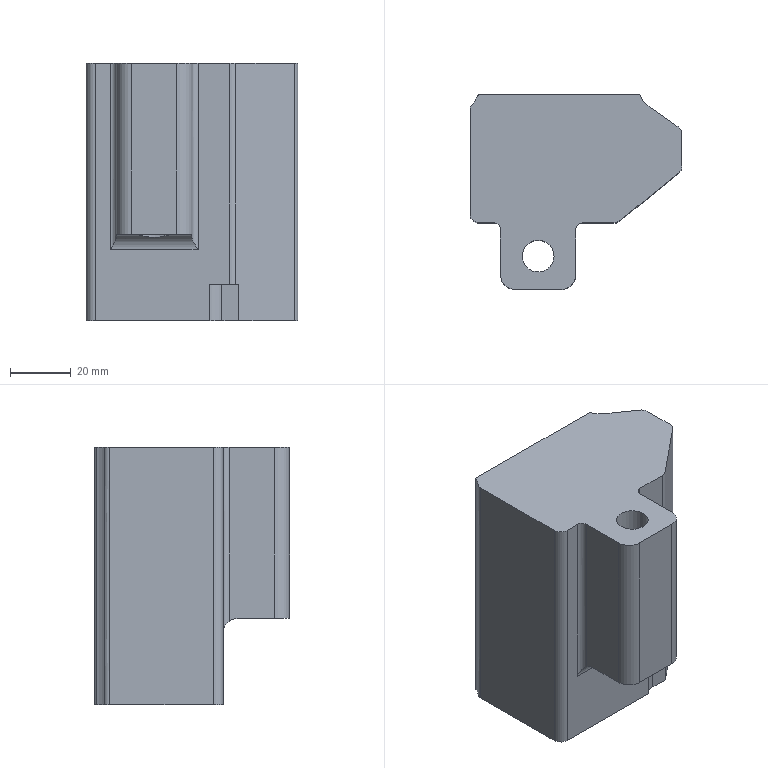Part | NX | features PU-14 2 | 1 solid | 32 faces | box 70 x 64.5 x 85 mm | volume 251895 mm3 | cylinder 16 | plane 15 | spline 1 | commonest cylinder face diameters 6 x4 10 x4 2 x2 4 x2 10.5 x1 16 x1
STEP:
#1=CARTESIAN_POINT('',(3938.531,-860.622,860.716));
#2=VERTEX_POINT('',#1);
#3=CARTESIAN_POINT('',(3990.637,-860.622,860.716));
#4=VERTEX_POINT('',#3);
#5=CARTESIAN_POINT('',(3980.707,-860.622,860.716));
#6=DIRECTION('',(1.,0.,0.));
#7=VECTOR('',#6,1000.);
#8=LINE('',#5,#7);
#9=EDGE_CURVE('',#2,#4,#8,.T.);
#10=ORIENTED_EDGE('',*,*,#9,.T.);
#11=CARTESIAN_POINT('',(3991.558,-861.233,860.716));
#12=VERTEX_POINT('',#11);
#13=CARTESIAN_POINT('',(3990.637,-861.622,860.716));
#14=DIRECTION('',(0.,-0.000000114,-1.));
#15=DIRECTION('',(0.,1.,-0.000000114));
#16=AXIS2_PLACEMENT_3D('',#13,#14,#15);
#17=CIRCLE('',#16,1.);
#18=EDGE_CURVE('',#4,#12,#17,.T.);
#19=ORIENTED_EDGE('',*,*,#18,.T.);
#20=CARTESIAN_POINT('',(3994.365,-864.693,860.716));
#21=VERTEX_POINT('',#20);
#22=CARTESIAN_POINT('',(3998.929,-858.122,860.716));
#23=DIRECTION('',(0.,-0.000000114,-1.));
#24=DIRECTION('',(0.,1.,-0.000000114));
#25=AXIS2_PLACEMENT_3D('',#22,#23,#24);
#26=CIRCLE('',#25,8.);
#27=EDGE_CURVE('',#12,#21,#26,.F.);
#28=ORIENTED_EDGE('',*,*,#27,.T.);
#29=CARTESIAN_POINT('',(4003.948,-871.349,860.716));
#30=VERTEX_POINT('',#29);
#31=CARTESIAN_POINT('',(3973.171,-849.972,860.716));
#32=DIRECTION('',(-0.8213,0.5705,-0.000000065));
#33=VECTOR('',#32,1000.);
#34=LINE('',#31,#33);
#35=EDGE_CURVE('',#21,#30,#34,.F.);
#36=ORIENTED_EDGE('',*,*,#35,.T.);
#37=CARTESIAN_POINT('',(4005.236,-873.813,860.716));
#38=VERTEX_POINT('',#37);
#39=CARTESIAN_POINT('',(4002.236,-873.813,860.716));
#40=DIRECTION('',(0.,-0.000000114,-1.));
#41=DIRECTION('',(0.,1.,-0.000000114));
#42=AXIS2_PLACEMENT_3D('',#39,#40,#41);
#43=CIRCLE('',#42,3.);
#44=EDGE_CURVE('',#30,#38,#43,.T.);
#45=ORIENTED_EDGE('',*,*,#44,.T.);
#46=CARTESIAN_POINT('',(4005.236,-884.324,860.716));
#47=VERTEX_POINT('',#46);
#48=CARTESIAN_POINT('',(4005.236,-838.813,860.716));
#49=DIRECTION('',(0.,1.,-0.000000114));
#50=VECTOR('',#49,1000.);
#51=LINE('',#48,#50);
#52=EDGE_CURVE('',#47,#38,#51,.T.);
#53=ORIENTED_EDGE('',*,*,#52,.F.);
#54=CARTESIAN_POINT('',(4004.128,-886.652,860.716));
#55=VERTEX_POINT('',#54);
#56=CARTESIAN_POINT('',(4002.236,-884.324,860.716));
#57=DIRECTION('',(0.,-0.000000114,-1.));
#58=DIRECTION('',(0.,1.,-0.000000114));
#59=AXIS2_PLACEMENT_3D('',#56,#57,#58);
#60=CIRCLE('',#59,3.);
#61=EDGE_CURVE('',#47,#55,#60,.T.);
#62=ORIENTED_EDGE('',*,*,#61,.T.);
#63=CARTESIAN_POINT('',(3985.708,-901.619,860.716));
#64=VERTEX_POINT('',#63);
#65=CARTESIAN_POINT('',(3999.843,-890.134,860.716));
#66=DIRECTION('',(0.7761,0.6306,-0.000000072));
#67=VECTOR('',#66,1000.);
#68=LINE('',#65,#67);
#69=EDGE_CURVE('',#64,#55,#68,.T.);
#70=ORIENTED_EDGE('',*,*,#69,.F.);
#71=CARTESIAN_POINT('',(3980.105,-901.423,860.716));
#72=VERTEX_POINT('',#71);
#73=CARTESIAN_POINT('',(3978.533,-901.368,860.716));
#74=DIRECTION('',(-0.9994,0.0349,-0.000000004));
#75=VECTOR('',#74,1000.);
#76=LINE('',#73,#75);
#77=EDGE_CURVE('',#64,#72,#76,.T.);
#78=ORIENTED_EDGE('',*,*,#77,.T.);
#79=CARTESIAN_POINT('',(3976.172,-903.122,860.716));
#80=VERTEX_POINT('',#79);
#81=CARTESIAN_POINT('',(3979.931,-906.42,860.716));
#82=DIRECTION('',(0.,-0.000000114,-1.));
#83=DIRECTION('',(0.,1.,-0.000000114));
#84=AXIS2_PLACEMENT_3D('',#81,#82,#83);
#85=CIRCLE('',#84,5.);
#86=EDGE_CURVE('',#80,#72,#85,.T.);
#87=ORIENTED_EDGE('',*,*,#86,.F.);
#88=CARTESIAN_POINT('',(3938.236,-903.122,860.716));
#89=VERTEX_POINT('',#88);
#90=CARTESIAN_POINT('',(3980.707,-903.122,860.716));
#91=DIRECTION('',(1.,0.,0.));
#92=VECTOR('',#91,1000.);
#93=LINE('',#90,#92);
#94=EDGE_CURVE('',#89,#80,#93,.T.);
#95=ORIENTED_EDGE('',*,*,#94,.F.);
#96=CARTESIAN_POINT('',(3935.236,-900.122,860.716));
#97=VERTEX_POINT('',#96);
#98=CARTESIAN_POINT('',(3938.236,-900.122,860.716));
#99=DIRECTION('',(0.,-0.000000114,-1.));
#100=DIRECTION('',(0.,1.,-0.000000114));
#101=AXIS2_PLACEMENT_3D('',#98,#99,#100);
#102=CIRCLE('',#101,3.);
#103=EDGE_CURVE('',#89,#97,#102,.T.);
#104=ORIENTED_EDGE('',*,*,#103,.T.);
#105=CARTESIAN_POINT('',(3935.236,-896.605,860.716));
#106=VERTEX_POINT('',#105);
#107=CARTESIAN_POINT('',(3935.236,-839.123,860.716));
#108=DIRECTION('',(0.,1.,-0.000000114));
#109=VECTOR('',#108,1000.);
#110=LINE('',#107,#109);
#111=EDGE_CURVE('',#97,#106,#110,.T.);
#112=ORIENTED_EDGE('',*,*,#111,.T.);
#113=CARTESIAN_POINT('',(3935.236,-865.633,860.716));
#114=VERTEX_POINT('',#113);
#115=CARTESIAN_POINT('',(3935.236,-839.123,860.716));
#116=DIRECTION('',(0.,1.,-0.000000114));
#117=VECTOR('',#116,1000.);
#118=LINE('',#115,#117);
#119=EDGE_CURVE('',#106,#114,#118,.T.);
#120=ORIENTED_EDGE('',*,*,#119,.T.);
#121=CARTESIAN_POINT('',(3935.909,-863.926,860.716));
#122=VERTEX_POINT('',#121);
#123=CARTESIAN_POINT('',(3937.736,-865.633,860.716));
#124=DIRECTION('',(0.,-0.000000114,-1.));
#125=DIRECTION('',(0.,1.,-0.000000114));
#126=AXIS2_PLACEMENT_3D('',#123,#124,#125);
#127=CIRCLE('',#126,2.5);
#128=EDGE_CURVE('',#114,#122,#127,.T.);
#129=ORIENTED_EDGE('',*,*,#128,.T.);
#130=CARTESIAN_POINT('',(3937.601,-861.254,860.716));
#131=VERTEX_POINT('',#130);
#132=CARTESIAN_POINT('',(3929.699,-858.122,860.716));
#133=DIRECTION('',(0.,-0.000000114,-1.));
#134=DIRECTION('',(0.,1.,-0.000000114));
#135=AXIS2_PLACEMENT_3D('',#132,#133,#134);
#136=CIRCLE('',#135,8.5);
#137=EDGE_CURVE('',#122,#131,#136,.F.);
#138=ORIENTED_EDGE('',*,*,#137,.T.);
#139=CARTESIAN_POINT('',(3938.531,-861.622,860.716));
#140=DIRECTION('',(0.,-0.000000114,-1.));
#141=DIRECTION('',(0.,1.,-0.000000114));
#142=AXIS2_PLACEMENT_3D('',#139,#140,#141);
#143=CIRCLE('',#142,1.);
#144=EDGE_CURVE('',#131,#2,#143,.T.);
#145=ORIENTED_EDGE('',*,*,#144,.T.);
#146=EDGE_LOOP('',(#10,#19,#28,#36,#45,#53,#62,#70,#78,#87,#95,#104,#112,#120,#129,#138,#145));
#147=FACE_BOUND('',#146,.T.);
#148=CARTESIAN_POINT('',(3980.707,-839.123,860.716));
#149=DIRECTION('',(0.,-0.000000114,-1.));
#150=DIRECTION('',(0.,-1.,0.000000114));
#151=AXIS2_PLACEMENT_3D('',#148,#149,#150);
#152=PLANE('',#151);
#153=ADVANCED_FACE('',(#147),#152,.T.);
#154=ORIENTED_EDGE('',*,*,#27,.F.);
#155=CARTESIAN_POINT('',(3991.558,-861.233,945.716));
#156=VERTEX_POINT('',#155);
#157=CARTESIAN_POINT('',(3991.558,-861.233,859.72));
#158=DIRECTION('',(0.,0.,-1.));
#159=VECTOR('',#158,1000.);
#160=LINE('',#157,#159);
#161=EDGE_CURVE('',#12,#156,#160,.F.);
#162=ORIENTED_EDGE('',*,*,#161,.T.);
#163=CARTESIAN_POINT('',(3994.365,-864.693,945.716));
#164=VERTEX_POINT('',#163);
#165=CARTESIAN_POINT('',(3998.929,-858.122,945.716));
#166=DIRECTION('',(0.,0.,1.));
#167=DIRECTION('',(1.,0.,0.));
#168=AXIS2_PLACEMENT_3D('',#165,#166,#167);
#169=CIRCLE('',#168,8.);
#170=EDGE_CURVE('',#164,#156,#169,.F.);
#171=ORIENTED_EDGE('',*,*,#170,.F.);
#172=CARTESIAN_POINT('',(3994.365,-864.693,935.716));
#173=DIRECTION('',(0.,0.,1.));
#174=VECTOR('',#173,1000.);
#175=LINE('',#172,#174);
#176=EDGE_CURVE('',#21,#164,#175,.T.);
#177=ORIENTED_EDGE('',*,*,#176,.F.);
#178=EDGE_LOOP('',(#154,#162,#171,#177));
#179=FACE_BOUND('',#178,.T.);
#180=CARTESIAN_POINT('',(3998.929,-858.122,859.72));
#181=DIRECTION('',(0.,0.,-1.));
#182=DIRECTION('',(-1.,0.,0.));
#183=AXIS2_PLACEMENT_3D('',#180,#181,#182);
#184=CYLINDRICAL_SURFACE('',#183,8.);
#185=ADVANCED_FACE('',(#179),#184,.F.);
#186=CARTESIAN_POINT('',(3937.601,-861.254,945.716));
#187=VERTEX_POINT('',#186);
#188=CARTESIAN_POINT('',(3935.909,-863.926,945.716));
#189=VERTEX_POINT('',#188);
#190=CARTESIAN_POINT('',(3929.699,-858.122,945.716));
#191=DIRECTION('',(0.,0.,1.));
#192=DIRECTION('',(1.,0.,0.));
#193=AXIS2_PLACEMENT_3D('',#190,#191,#192);
#194=CIRCLE('',#193,8.5);
#195=EDGE_CURVE('',#187,#189,#194,.F.);
#196=ORIENTED_EDGE('',*,*,#195,.F.);
#197=CARTESIAN_POINT('',(3937.601,-861.254,889.216));
#198=DIRECTION('',(0.,0.,-1.));
#199=VECTOR('',#198,1000.);
#200=LINE('',#197,#199);
#201=EDGE_CURVE('',#187,#131,#200,.T.);
#202=ORIENTED_EDGE('',*,*,#201,.T.);
#203=ORIENTED_EDGE('',*,*,#137,.F.);
#204=CARTESIAN_POINT('',(3935.909,-863.926,860.716));
#205=CARTESIAN_POINT('',(3935.909,-863.926,889.05));
#206=CARTESIAN_POINT('',(3935.909,-863.926,917.383));
#207=CARTESIAN_POINT('',(3935.909,-863.926,945.716));
#208=B_SPLINE_CURVE_WITH_KNOTS('',3,(#204,#205,#206,#207),.UNSPECIFIED.,.F.,.F.,(4,4),(0.,0.085),.UNSPECIFIED.);
#209=EDGE_CURVE('',#122,#189,#208,.T.);
#210=ORIENTED_EDGE('',*,*,#209,.T.);
#211=EDGE_LOOP('',(#196,#202,#203,#210));
#212=FACE_BOUND('',#211,.T.);
#213=CARTESIAN_POINT('',(3929.699,-858.122,889.216));
#214=DIRECTION('',(0.,0.,-1.));
#215=DIRECTION('',(-1.,0.,0.));
#216=AXIS2_PLACEMENT_3D('',#213,#214,#215);
#217=CYLINDRICAL_SURFACE('',#216,8.5);
#218=ADVANCED_FACE('',(#212),#217,.F.);
#219=CARTESIAN_POINT('',(3962.986,-914.122,945.716));
#220=VERTEX_POINT('',#219);
#221=CARTESIAN_POINT('',(3957.736,-914.122,945.716));
#222=DIRECTION('',(0.,0.,1.));
#223=DIRECTION('',(1.,0.,0.));
#224=AXIS2_PLACEMENT_3D('',#221,#222,#223);
#225=CIRCLE('',#224,5.25);
#226=EDGE_CURVE('',#220,#220,#225,.F.);
#227=ORIENTED_EDGE('',*,*,#226,.T.);
#228=EDGE_LOOP('',(#227));
#229=FACE_BOUND('',#228,.T.);
#230=ORIENTED_EDGE('',*,*,#170,.T.);
#231=CARTESIAN_POINT('',(3990.637,-860.622,945.716));
#232=VERTEX_POINT('',#231);
#233=CARTESIAN_POINT('',(3990.637,-861.622,945.716));
#234=DIRECTION('',(0.,0.,1.));
#235=DIRECTION('',(1.,0.,0.));
#236=AXIS2_PLACEMENT_3D('',#233,#234,#235);
#237=CIRCLE('',#236,1.);
#238=EDGE_CURVE('',#156,#232,#237,.T.);
#239=ORIENTED_EDGE('',*,*,#238,.T.);
#240=CARTESIAN_POINT('',(3938.531,-860.622,945.716));
#241=VERTEX_POINT('',#240);
#242=CARTESIAN_POINT('',(3512.919,-860.622,945.716));
#243=DIRECTION('',(-1.,0.,0.));
#244=VECTOR('',#243,1000.);
#245=LINE('',#242,#244);
#246=EDGE_CURVE('',#232,#241,#245,.T.);
#247=ORIENTED_EDGE('',*,*,#246,.T.);
#248=CARTESIAN_POINT('',(3938.531,-861.622,945.716));
#249=DIRECTION('',(0.,0.,1.));
#250=DIRECTION('',(1.,0.,0.));
#251=AXIS2_PLACEMENT_3D('',#248,#249,#250);
#252=CIRCLE('',#251,1.);
#253=EDGE_CURVE('',#241,#187,#252,.T.);
#254=ORIENTED_EDGE('',*,*,#253,.T.);
#255=ORIENTED_EDGE('',*,*,#195,.T.);
#256=CARTESIAN_POINT('',(3935.236,-865.633,945.716));
#257=VERTEX_POINT('',#256);
#258=CARTESIAN_POINT('',(3937.736,-865.633,945.716));
#259=DIRECTION('',(0.,0.,1.));
#260=DIRECTION('',(1.,0.,0.));
#261=AXIS2_PLACEMENT_3D('',#258,#259,#260);
#262=CIRCLE('',#261,2.5);
#263=EDGE_CURVE('',#189,#257,#262,.T.);
#264=ORIENTED_EDGE('',*,*,#263,.T.);
#265=CARTESIAN_POINT('',(3935.236,-900.122,945.716));
#266=VERTEX_POINT('',#265);
#267=CARTESIAN_POINT('',(3935.236,-911.724,945.716));
#268=DIRECTION('',(0.,-1.,0.));
#269=VECTOR('',#268,1000.);
#270=LINE('',#267,#269);
#271=EDGE_CURVE('',#266,#257,#270,.F.);
#272=ORIENTED_EDGE('',*,*,#271,.F.);
#273=CARTESIAN_POINT('',(3938.236,-903.122,945.716));
#274=VERTEX_POINT('',#273);
#275=CARTESIAN_POINT('',(3938.236,-900.122,945.716));
#276=DIRECTION('',(0.,0.,1.));
#277=DIRECTION('',(1.,0.,0.));
#278=AXIS2_PLACEMENT_3D('',#275,#276,#277);
#279=CIRCLE('',#278,3.);
#280=EDGE_CURVE('',#266,#274,#279,.T.);
#281=ORIENTED_EDGE('',*,*,#280,.T.);
#282=CARTESIAN_POINT('',(3943.236,-903.122,945.716));
#283=VERTEX_POINT('',#282);
#284=CARTESIAN_POINT('',(3512.919,-903.122,945.716));
#285=DIRECTION('',(-1.,0.,0.));
#286=VECTOR('',#285,1000.);
#287=LINE('',#284,#286);
#288=EDGE_CURVE('',#274,#283,#287,.F.);
#289=ORIENTED_EDGE('',*,*,#288,.T.);
#290=CARTESIAN_POINT('',(3945.236,-905.122,945.716));
#291=VERTEX_POINT('',#290);
#292=CARTESIAN_POINT('',(3943.236,-905.122,945.716));
#293=DIRECTION('',(0.,0.,1.));
#294=DIRECTION('',(1.,0.,0.));
#295=AXIS2_PLACEMENT_3D('',#292,#293,#294);
#296=CIRCLE('',#295,2.);
#297=EDGE_CURVE('',#283,#291,#296,.F.);
#298=ORIENTED_EDGE('',*,*,#297,.T.);
#299=CARTESIAN_POINT('',(3945.236,-920.122,945.716));
#300=VERTEX_POINT('',#299);
#301=CARTESIAN_POINT('',(3945.236,-903.122,945.716));
#302=DIRECTION('',(0.,1.,0.));
#303=VECTOR('',#302,1000.);
#304=LINE('',#301,#303);
#305=EDGE_CURVE('',#291,#300,#304,.F.);
#306=ORIENTED_EDGE('',*,*,#305,.T.);
#307=CARTESIAN_POINT('',(3950.236,-925.122,945.716));
#308=VERTEX_POINT('',#307);
#309=CARTESIAN_POINT('',(3950.236,-920.122,945.716));
#310=DIRECTION('',(0.,0.,-1.));
#311=DIRECTION('',(-1.,0.,0.));
#312=AXIS2_PLACEMENT_3D('',#309,#310,#311);
#313=CIRCLE('',#312,5.);
#314=EDGE_CURVE('',#300,#308,#313,.F.);
#315=ORIENTED_EDGE('',*,*,#314,.T.);
#316=CARTESIAN_POINT('',(3965.236,-925.122,945.716));
#317=VERTEX_POINT('',#316);
#318=CARTESIAN_POINT('',(3512.919,-925.122,945.716));
#319=DIRECTION('',(1.,0.,0.));
#320=VECTOR('',#319,1000.);
#321=LINE('',#318,#320);
#322=EDGE_CURVE('',#308,#317,#321,.T.);
#323=ORIENTED_EDGE('',*,*,#322,.T.);
#324=CARTESIAN_POINT('',(3970.236,-920.122,945.716));
#325=VERTEX_POINT('',#324);
#326=CARTESIAN_POINT('',(3965.236,-920.122,945.716));
#327=DIRECTION('',(0.,0.,-1.));
#328=DIRECTION('',(-1.,0.,0.));
#329=AXIS2_PLACEMENT_3D('',#326,#327,#328);
#330=CIRCLE('',#329,5.);
#331=EDGE_CURVE('',#317,#325,#330,.F.);
#332=ORIENTED_EDGE('',*,*,#331,.T.);
#333=CARTESIAN_POINT('',(3970.236,-905.122,945.716));
#334=VERTEX_POINT('',#333);
#335=CARTESIAN_POINT('',(3970.236,-903.122,945.716));
#336=DIRECTION('',(0.,1.,0.));
#337=VECTOR('',#336,1000.);
#338=LINE('',#335,#337);
#339=EDGE_CURVE('',#334,#325,#338,.F.);
#340=ORIENTED_EDGE('',*,*,#339,.F.);
#341=CARTESIAN_POINT('',(3972.236,-903.122,945.716));
#342=VERTEX_POINT('',#341);
#343=CARTESIAN_POINT('',(3972.236,-905.122,945.716));
#344=DIRECTION('',(0.,0.,1.));
#345=DIRECTION('',(1.,0.,0.));
#346=AXIS2_PLACEMENT_3D('',#343,#344,#345);
#347=CIRCLE('',#346,2.);
#348=EDGE_CURVE('',#334,#342,#347,.F.);
#349=ORIENTED_EDGE('',*,*,#348,.T.);
#350=CARTESIAN_POINT('',(3982.792,-903.122,945.716));
#351=VERTEX_POINT('',#350);
#352=CARTESIAN_POINT('',(3512.919,-903.122,945.716));
#353=DIRECTION('',(-1.,0.,0.));
#354=VECTOR('',#353,1000.);
#355=LINE('',#352,#354);
#356=EDGE_CURVE('',#342,#351,#355,.F.);
#357=ORIENTED_EDGE('',*,*,#356,.T.);
#358=CARTESIAN_POINT('',(3984.684,-902.451,945.716));
#359=VERTEX_POINT('',#358);
#360=CARTESIAN_POINT('',(3982.792,-900.122,945.716));
#361=DIRECTION('',(0.,0.,1.));
#362=DIRECTION('',(1.,0.,0.));
#363=AXIS2_PLACEMENT_3D('',#360,#361,#362);
#364=CIRCLE('',#363,3.);
#365=EDGE_CURVE('',#359,#351,#364,.F.);
#366=ORIENTED_EDGE('',*,*,#365,.F.);
#367=CARTESIAN_POINT('',(4004.128,-886.652,945.716));
#368=VERTEX_POINT('',#367);
#369=CARTESIAN_POINT('',(3695.977,-1137.025,945.716));
#370=DIRECTION('',(0.7761,0.6306,0.));
#371=VECTOR('',#370,1000.);
#372=LINE('',#369,#371);
#373=EDGE_CURVE('',#368,#359,#372,.F.);
#374=ORIENTED_EDGE('',*,*,#373,.F.);
#375=CARTESIAN_POINT('',(4005.236,-884.324,945.716));
#376=VERTEX_POINT('',#375);
#377=CARTESIAN_POINT('',(4002.236,-884.324,945.716));
#378=DIRECTION('',(0.,0.,1.));
#379=DIRECTION('',(1.,0.,0.));
#380=AXIS2_PLACEMENT_3D('',#377,#378,#379);
#381=CIRCLE('',#380,3.);
#382=EDGE_CURVE('',#376,#368,#381,.F.);
#383=ORIENTED_EDGE('',*,*,#382,.F.);
#384=CARTESIAN_POINT('',(4005.236,-873.813,945.716));
#385=VERTEX_POINT('',#384);
#386=CARTESIAN_POINT('',(4005.236,-911.724,945.716));
#387=DIRECTION('',(0.,1.,0.));
#388=VECTOR('',#387,1000.);
#389=LINE('',#386,#388);
#390=EDGE_CURVE('',#385,#376,#389,.F.);
#391=ORIENTED_EDGE('',*,*,#390,.F.);
#392=CARTESIAN_POINT('',(4003.948,-871.349,945.716));
#393=VERTEX_POINT('',#392);
#394=CARTESIAN_POINT('',(4002.236,-873.813,945.716));
#395=DIRECTION('',(0.,0.,1.));
#396=DIRECTION('',(1.,0.,0.));
#397=AXIS2_PLACEMENT_3D('',#394,#395,#396);
#398=CIRCLE('',#397,3.);
#399=EDGE_CURVE('',#393,#385,#398,.F.);
#400=ORIENTED_EDGE('',*,*,#399,.F.);
#401=CARTESIAN_POINT('',(3996.884,-866.442,945.716));
#402=DIRECTION('',(0.8213,-0.5705,0.));
#403=VECTOR('',#402,1000.);
#404=LINE('',#401,#403);
#405=EDGE_CURVE('',#164,#393,#404,.T.);
#406=ORIENTED_EDGE('',*,*,#405,.F.);
#407=EDGE_LOOP('',(#230,#239,#247,#254,#255,#264,#272,#281,#289,#298,#306,#315,#323,#332,#340,#349,#357,#366,#374,#383,#391,#400,#406));
#408=FACE_BOUND('',#407,.T.);
#409=CARTESIAN_POINT('',(3512.919,-911.724,945.716));
#410=DIRECTION('',(0.,0.,1.));
#411=DIRECTION('',(1.,0.,0.));
#412=AXIS2_PLACEMENT_3D('',#409,#410,#411);
#413=PLANE('',#412);
#414=ADVANCED_FACE('',(#229,#408),#413,.T.);
#415=CARTESIAN_POINT('',(3985.708,-901.619,872.698));
#416=VERTEX_POINT('',#415);
#417=CARTESIAN_POINT('',(3985.708,-901.619,859.716));
#418=DIRECTION('',(0.,0.,-1.));
#419=VECTOR('',#418,1000.);
#420=LINE('',#417,#419);
#421=EDGE_CURVE('',#416,#64,#420,.T.);
#422=ORIENTED_EDGE('',*,*,#421,.F.);
#423=CARTESIAN_POINT('',(3980.105,-901.423,872.698));
#424=VERTEX_POINT('',#423);
#425=CARTESIAN_POINT('',(3972.779,-901.167,872.698));
#426=DIRECTION('',(-0.9994,0.0349,-0.000000001));
#427=VECTOR('',#426,1000.);
#428=LINE('',#425,#427);
#429=EDGE_CURVE('',#416,#424,#428,.T.);
#430=ORIENTED_EDGE('',*,*,#429,.T.);
#431=CARTESIAN_POINT('',(3980.105,-901.423,820.698));
#432=DIRECTION('',(0.,0.,1.));
#433=VECTOR('',#432,1000.);
#434=LINE('',#431,#433);
#435=EDGE_CURVE('',#424,#72,#434,.F.);
#436=ORIENTED_EDGE('',*,*,#435,.T.);
#437=ORIENTED_EDGE('',*,*,#77,.F.);
#438=EDGE_LOOP('',(#422,#430,#436,#437));
#439=FACE_BOUND('',#438,.T.);
#440=CARTESIAN_POINT('',(3972.779,-901.167,820.698));
#441=DIRECTION('',(-0.0349,-0.9994,0.));
#442=DIRECTION('',(0.9994,-0.0349,0.));
#443=AXIS2_PLACEMENT_3D('',#440,#441,#442);
#444=PLANE('',#443);
#445=ADVANCED_FACE('',(#439),#444,.T.);
#446=ORIENTED_EDGE('',*,*,#176,.T.);
#447=ORIENTED_EDGE('',*,*,#405,.T.);
#448=CARTESIAN_POINT('',(4003.948,-871.349,859.72));
#449=DIRECTION('',(0.,0.,-1.));
#450=VECTOR('',#449,1000.);
#451=LINE('',#448,#450);
#452=EDGE_CURVE('',#30,#393,#451,.F.);
#453=ORIENTED_EDGE('',*,*,#452,.F.);
#454=ORIENTED_EDGE('',*,*,#35,.F.);
#455=EDGE_LOOP('',(#446,#447,#453,#454));
#456=FACE_BOUND('',#455,.T.);
#457=CARTESIAN_POINT('',(3996.884,-866.442,859.72));
#458=DIRECTION('',(-0.5705,-0.8213,0.));
#459=DIRECTION('',(0.8213,-0.5705,0.));
#460=AXIS2_PLACEMENT_3D('',#457,#458,#459);
#461=PLANE('',#460);
#462=ADVANCED_FACE('',(#456),#461,.F.);
#463=CARTESIAN_POINT('',(3972.236,-903.122,884.217));
#464=VERTEX_POINT('',#463);
#465=CARTESIAN_POINT('',(3943.236,-903.122,884.217));
#466=VERTEX_POINT('',#465);
#467=CARTESIAN_POINT('',(3938.199,-903.122,884.217));
#468=DIRECTION('',(-1.,0.,0.));
#469=VECTOR('',#468,1000.);
#470=LINE('',#467,#469);
#471=EDGE_CURVE('',#464,#466,#470,.T.);
#472=ORIENTED_EDGE('',*,*,#471,.T.);
#473=CARTESIAN_POINT('',(3943.236,-903.122,860.716));
#474=DIRECTION('',(0.,0.,-1.));
#475=VECTOR('',#474,1000.);
#476=LINE('',#473,#475);
#477=EDGE_CURVE('',#466,#283,#476,.F.);
#478=ORIENTED_EDGE('',*,*,#477,.T.);
#479=ORIENTED_EDGE('',*,*,#288,.F.);
#480=CARTESIAN_POINT('',(3938.236,-903.122,860.716));
#481=DIRECTION('',(0.,0.,-1.));
#482=VECTOR('',#481,1000.);
#483=LINE('',#480,#482);
#484=EDGE_CURVE('',#274,#89,#483,.T.);
#485=ORIENTED_EDGE('',*,*,#484,.T.);
#486=ORIENTED_EDGE('',*,*,#94,.T.);
#487=CARTESIAN_POINT('',(3976.172,-903.122,872.698));
#488=VERTEX_POINT('',#487);
#489=CARTESIAN_POINT('',(3976.172,-903.122,866.707));
#490=DIRECTION('',(0.,0.,1.));
#491=VECTOR('',#490,1000.);
#492=LINE('',#489,#491);
#493=EDGE_CURVE('',#80,#488,#492,.T.);
#494=ORIENTED_EDGE('',*,*,#493,.T.);
#495=CARTESIAN_POINT('',(3982.792,-903.122,872.698));
#496=VERTEX_POINT('',#495);
#497=CARTESIAN_POINT('',(3938.199,-903.122,872.698));
#498=DIRECTION('',(1.,0.,0.000000001));
#499=VECTOR('',#498,1000.);
#500=LINE('',#497,#499);
#501=EDGE_CURVE('',#488,#496,#500,.T.);
#502=ORIENTED_EDGE('',*,*,#501,.T.);
#503=CARTESIAN_POINT('',(3982.792,-903.122,860.716));
#504=DIRECTION('',(0.,0.,1.));
#505=VECTOR('',#504,1000.);
#506=LINE('',#503,#505);
#507=EDGE_CURVE('',#351,#496,#506,.F.);
#508=ORIENTED_EDGE('',*,*,#507,.F.);
#509=ORIENTED_EDGE('',*,*,#356,.F.);
#510=CARTESIAN_POINT('',(3972.236,-903.122,894.217));
#511=DIRECTION('',(0.,0.,1.));
#512=VECTOR('',#511,1000.);
#513=LINE('',#510,#512);
#514=EDGE_CURVE('',#342,#464,#513,.F.);
#515=ORIENTED_EDGE('',*,*,#514,.T.);
#516=EDGE_LOOP('',(#472,#478,#479,#485,#486,#494,#502,#508,#509,#515));
#517=FACE_BOUND('',#516,.T.);
#518=CARTESIAN_POINT('',(3938.199,-903.122,860.716));
#519=DIRECTION('',(0.,1.,0.));
#520=DIRECTION('',(0.,0.,1.));
#521=AXIS2_PLACEMENT_3D('',#518,#519,#520);
#522=PLANE('',#521);
#523=ADVANCED_FACE('',(#517),#522,.F.);
#524=ORIENTED_EDGE('',*,*,#484,.F.);
#525=ORIENTED_EDGE('',*,*,#280,.F.);
#526=CARTESIAN_POINT('',(3935.236,-900.122,860.716));
#527=DIRECTION('',(0.,0.,-1.));
#528=VECTOR('',#527,1000.);
#529=LINE('',#526,#528);
#530=EDGE_CURVE('',#97,#266,#529,.F.);
#531=ORIENTED_EDGE('',*,*,#530,.F.);
#532=ORIENTED_EDGE('',*,*,#103,.F.);
#533=EDGE_LOOP('',(#524,#525,#531,#532));
#534=FACE_BOUND('',#533,.T.);
#535=CARTESIAN_POINT('',(3938.236,-900.122,860.716));
#536=DIRECTION('',(0.,0.,1.));
#537=DIRECTION('',(1.,0.,0.));
#538=AXIS2_PLACEMENT_3D('',#535,#536,#537);
#539=CYLINDRICAL_SURFACE('',#538,3.);
#540=ADVANCED_FACE('',(#534),#539,.T.);
#541=CARTESIAN_POINT('',(3935.236,-865.633,945.716));
#542=CARTESIAN_POINT('',(3935.236,-865.633,917.383));
#543=CARTESIAN_POINT('',(3935.236,-865.633,889.05));
#544=CARTESIAN_POINT('',(3935.236,-865.633,860.716));
#545=B_SPLINE_CURVE_WITH_KNOTS('',3,(#541,#542,#543,#544),.UNSPECIFIED.,.F.,.F.,(4,4),(-0.01,0.075),.UNSPECIFIED.);
#546=EDGE_CURVE('',#257,#114,#545,.T.);
#547=ORIENTED_EDGE('',*,*,#546,.F.);
#548=ORIENTED_EDGE('',*,*,#263,.F.);
#549=ORIENTED_EDGE('',*,*,#209,.F.);
#550=ORIENTED_EDGE('',*,*,#128,.F.);
#551=EDGE_LOOP('',(#547,#548,#549,#550));
#552=FACE_BOUND('',#551,.T.);
#553=CARTESIAN_POINT('',(3935.236,-865.633,860.716));
#554=CARTESIAN_POINT('',(3935.236,-864.646,860.716));
#555=CARTESIAN_POINT('',(3935.909,-863.926,860.716));
#556=CARTESIAN_POINT('',(3935.236,-865.633,889.05));
#557=CARTESIAN_POINT('',(3935.236,-864.646,889.05));
#558=CARTESIAN_POINT('',(3935.909,-863.926,889.05));
#559=CARTESIAN_POINT('',(3935.236,-865.633,917.383));
#560=CARTESIAN_POINT('',(3935.236,-864.646,917.383));
#561=CARTESIAN_POINT('',(3935.909,-863.926,917.383));
#562=CARTESIAN_POINT('',(3935.236,-865.633,945.716));
#563=CARTESIAN_POINT('',(3935.236,-864.646,945.716));
#564=CARTESIAN_POINT('',(3935.909,-863.926,945.716));
#565=(BOUNDED_SURFACE()B_SPLINE_SURFACE(3,2,((#553,#554,#555),(#556,#557,#558),(#559,#560,#561),(#562,#563,#564)),.UNSPECIFIED.,.F.,.F.,.F.)B_SPLINE_SURFACE_WITH_KNOTS((4,4),(3,3),(0.0725,0.1575),(0.,1.),.PIECEWISE_BEZIER_KNOTS.)GEOMETRIC_REPRESENTATION_ITEM()RATIONAL_B_SPLINE_SURFACE(((1.,0.9302,1.),(1.,0.9302,1.),(1.,0.9302,1.),(1.,0.9302,1.)))REPRESENTATION_ITEM('')SURFACE());
#566=ADVANCED_FACE('',(#552),#565,.T.);
#567=ORIENTED_EDGE('',*,*,#530,.T.);
#568=ORIENTED_EDGE('',*,*,#271,.T.);
#569=ORIENTED_EDGE('',*,*,#546,.T.);
#570=ORIENTED_EDGE('',*,*,#119,.F.);
#571=ORIENTED_EDGE('',*,*,#111,.F.);
#572=EDGE_LOOP('',(#567,#568,#569,#570,#571));
#573=FACE_BOUND('',#572,.T.);
#574=CARTESIAN_POINT('',(3935.236,-839.123,930.716));
#575=DIRECTION('',(-1.,0.,0.));
#576=DIRECTION('',(0.,0.000000114,1.));
#577=AXIS2_PLACEMENT_3D('',#574,#575,#576);
#578=PLANE('',#577);
#579=ADVANCED_FACE('',(#573),#578,.T.);
#580=CARTESIAN_POINT('',(3984.684,-902.451,872.698));
#581=VERTEX_POINT('',#580);
#582=CARTESIAN_POINT('',(3974.383,-910.82,872.698));
#583=DIRECTION('',(0.7761,0.6306,0.000000001));
#584=VECTOR('',#583,1000.);
#585=LINE('',#582,#584);
#586=EDGE_CURVE('',#581,#416,#585,.T.);
#587=ORIENTED_EDGE('',*,*,#586,.F.);
#588=CARTESIAN_POINT('',(3982.792,-900.122,872.698));
#589=DIRECTION('',(-0.000000001,0.,1.));
#590=DIRECTION('',(1.,0.,0.000000001));
#591=AXIS2_PLACEMENT_3D('',#588,#589,#590);
#592=CIRCLE('',#591,3.);
#593=EDGE_CURVE('',#581,#496,#592,.F.);
#594=ORIENTED_EDGE('',*,*,#593,.T.);
#595=ORIENTED_EDGE('',*,*,#501,.F.);
#596=CARTESIAN_POINT('',(3979.931,-906.42,872.698));
#597=DIRECTION('',(-0.000000001,0.,1.));
#598=DIRECTION('',(1.,0.,0.000000001));
#599=AXIS2_PLACEMENT_3D('',#596,#597,#598);
#600=CIRCLE('',#599,5.);
#601=EDGE_CURVE('',#488,#424,#600,.F.);
#602=ORIENTED_EDGE('',*,*,#601,.T.);
#603=ORIENTED_EDGE('',*,*,#429,.F.);
#604=EDGE_LOOP('',(#587,#594,#595,#602,#603));
#605=FACE_BOUND('',#604,.T.);
#606=CARTESIAN_POINT('',(3972.522,-908.529,872.698));
#607=DIRECTION('',(-0.000000001,0.,1.));
#608=DIRECTION('',(1.,0.,0.000000001));
#609=AXIS2_PLACEMENT_3D('',#606,#607,#608);
#610=PLANE('',#609);
#611=ADVANCED_FACE('',(#605),#610,.F.);
#612=ORIENTED_EDGE('',*,*,#86,.T.);
#613=ORIENTED_EDGE('',*,*,#435,.F.);
#614=ORIENTED_EDGE('',*,*,#601,.F.);
#615=ORIENTED_EDGE('',*,*,#493,.F.);
#616=EDGE_LOOP('',(#612,#613,#614,#615));
#617=FACE_BOUND('',#616,.T.);
#618=CARTESIAN_POINT('',(3979.931,-906.42,820.698));
#619=DIRECTION('',(0.,0.,1.));
#620=DIRECTION('',(1.,0.,0.));
#621=AXIS2_PLACEMENT_3D('',#618,#619,#620);
#622=CYLINDRICAL_SURFACE('',#621,5.);
#623=ADVANCED_FACE('',(#617),#622,.F.);
#624=CARTESIAN_POINT('',(3984.684,-902.451,859.716));
#625=DIRECTION('',(0.,0.,-1.));
#626=VECTOR('',#625,1000.);
#627=LINE('',#624,#626);
#628=EDGE_CURVE('',#359,#581,#627,.T.);
#629=ORIENTED_EDGE('',*,*,#628,.F.);
#630=ORIENTED_EDGE('',*,*,#365,.T.);
#631=ORIENTED_EDGE('',*,*,#507,.T.);
#632=ORIENTED_EDGE('',*,*,#593,.F.);
#633=EDGE_LOOP('',(#629,#630,#631,#632));
#634=FACE_BOUND('',#633,.T.);
#635=CARTESIAN_POINT('',(3982.792,-900.122,859.716));
#636=DIRECTION('',(0.,0.,1.));
#637=DIRECTION('',(1.,0.,0.));
#638=AXIS2_PLACEMENT_3D('',#635,#636,#637);
#639=CYLINDRICAL_SURFACE('',#638,3.);
#640=ADVANCED_FACE('',(#634),#639,.T.);
#641=CARTESIAN_POINT('',(4004.128,-886.652,910.716));
#642=DIRECTION('',(0.,0.,1.));
#643=VECTOR('',#642,1000.);
#644=LINE('',#641,#643);
#645=EDGE_CURVE('',#55,#368,#644,.T.);
#646=ORIENTED_EDGE('',*,*,#645,.T.);
#647=ORIENTED_EDGE('',*,*,#373,.T.);
#648=ORIENTED_EDGE('',*,*,#628,.T.);
#649=ORIENTED_EDGE('',*,*,#586,.T.);
#650=ORIENTED_EDGE('',*,*,#421,.T.);
#651=ORIENTED_EDGE('',*,*,#69,.T.);
#652=EDGE_LOOP('',(#646,#647,#648,#649,#650,#651));
#653=FACE_BOUND('',#652,.T.);
#654=CARTESIAN_POINT('',(3999.843,-890.134,859.716));
#655=DIRECTION('',(0.6306,-0.7761,0.));
#656=DIRECTION('',(0.7761,0.6306,0.));
#657=AXIS2_PLACEMENT_3D('',#654,#655,#656);
#658=PLANE('',#657);
#659=ADVANCED_FACE('',(#653),#658,.T.);
#660=CARTESIAN_POINT('',(4005.236,-884.324,935.716));
#661=DIRECTION('',(0.,0.,1.));
#662=VECTOR('',#661,1000.);
#663=LINE('',#660,#662);
#664=EDGE_CURVE('',#376,#47,#663,.F.);
#665=ORIENTED_EDGE('',*,*,#664,.F.);
#666=ORIENTED_EDGE('',*,*,#382,.T.);
#667=ORIENTED_EDGE('',*,*,#645,.F.);
#668=ORIENTED_EDGE('',*,*,#61,.F.);
#669=EDGE_LOOP('',(#665,#666,#667,#668));
#670=FACE_BOUND('',#669,.T.);
#671=CARTESIAN_POINT('',(4002.236,-884.324,930.716));
#672=DIRECTION('',(0.,0.,-1.));
#673=DIRECTION('',(-1.,0.,0.));
#674=AXIS2_PLACEMENT_3D('',#671,#672,#673);
#675=CYLINDRICAL_SURFACE('',#674,3.);
#676=ADVANCED_FACE('',(#670),#675,.T.);
#677=CARTESIAN_POINT('',(4005.236,-873.813,930.716));
#678=DIRECTION('',(0.,0.,-1.));
#679=VECTOR('',#678,1000.);
#680=LINE('',#677,#679);
#681=EDGE_CURVE('',#38,#385,#680,.F.);
#682=ORIENTED_EDGE('',*,*,#681,.T.);
#683=ORIENTED_EDGE('',*,*,#390,.T.);
#684=ORIENTED_EDGE('',*,*,#664,.T.);
#685=ORIENTED_EDGE('',*,*,#52,.T.);
#686=EDGE_LOOP('',(#682,#683,#684,#685));
#687=FACE_BOUND('',#686,.T.);
#688=CARTESIAN_POINT('',(4005.236,-838.813,930.716));
#689=DIRECTION('',(1.,0.,0.));
#690=DIRECTION('',(0.,-0.000000114,-1.));
#691=AXIS2_PLACEMENT_3D('',#688,#689,#690);
#692=PLANE('',#691);
#693=ADVANCED_FACE('',(#687),#692,.T.);
#694=ORIENTED_EDGE('',*,*,#452,.T.);
#695=ORIENTED_EDGE('',*,*,#399,.T.);
#696=ORIENTED_EDGE('',*,*,#681,.F.);
#697=ORIENTED_EDGE('',*,*,#44,.F.);
#698=EDGE_LOOP('',(#694,#695,#696,#697));
#699=FACE_BOUND('',#698,.T.);
#700=CARTESIAN_POINT('',(4002.236,-873.813,930.716));
#701=DIRECTION('',(0.,0.,-1.));
#702=DIRECTION('',(-1.,0.,0.));
#703=AXIS2_PLACEMENT_3D('',#700,#701,#702);
#704=CYLINDRICAL_SURFACE('',#703,3.);
#705=ADVANCED_FACE('',(#699),#704,.T.);
#706=CARTESIAN_POINT('',(3945.236,-920.122,889.217));
#707=VERTEX_POINT('',#706);
#708=CARTESIAN_POINT('',(3945.236,-908.122,889.217));
#709=VERTEX_POINT('',#708);
#710=CARTESIAN_POINT('',(3945.236,-772.636,889.217));
#711=DIRECTION('',(0.,1.,0.));
#712=VECTOR('',#711,1000.);
#713=LINE('',#710,#712);
#714=EDGE_CURVE('',#707,#709,#713,.T.);
#715=ORIENTED_EDGE('',*,*,#714,.T.);
#716=CARTESIAN_POINT('',(3951.028,-908.122,889.217));
#717=VERTEX_POINT('',#716);
#718=CARTESIAN_POINT('',(3804.403,-908.122,889.217));
#719=DIRECTION('',(-1.,0.,0.));
#720=VECTOR('',#719,1000.);
#721=LINE('',#718,#720);
#722=EDGE_CURVE('',#709,#717,#721,.F.);
#723=ORIENTED_EDGE('',*,*,#722,.T.);
#724=CARTESIAN_POINT('',(3964.444,-908.122,889.217));
#725=VERTEX_POINT('',#724);
#726=CARTESIAN_POINT('',(3957.736,-914.122,889.217));
#727=DIRECTION('',(0.,0.,-1.));
#728=DIRECTION('',(-1.,0.,0.));
#729=AXIS2_PLACEMENT_3D('',#726,#727,#728);
#730=CIRCLE('',#729,9.);
#731=EDGE_CURVE('',#725,#717,#730,.T.);
#732=ORIENTED_EDGE('',*,*,#731,.F.);
#733=CARTESIAN_POINT('',(3970.236,-908.122,889.217));
#734=VERTEX_POINT('',#733);
#735=CARTESIAN_POINT('',(3804.403,-908.122,889.217));
#736=DIRECTION('',(-1.,0.,0.));
#737=VECTOR('',#736,1000.);
#738=LINE('',#735,#737);
#739=EDGE_CURVE('',#725,#734,#738,.F.);
#740=ORIENTED_EDGE('',*,*,#739,.T.);
#741=CARTESIAN_POINT('',(3970.236,-920.122,889.217));
#742=VERTEX_POINT('',#741);
#743=CARTESIAN_POINT('',(3970.236,-772.636,889.217));
#744=DIRECTION('',(0.,1.,0.));
#745=VECTOR('',#744,1000.);
#746=LINE('',#743,#745);
#747=EDGE_CURVE('',#742,#734,#746,.T.);
#748=ORIENTED_EDGE('',*,*,#747,.F.);
#749=CARTESIAN_POINT('',(3965.236,-925.122,889.217));
#750=VERTEX_POINT('',#749);
#751=CARTESIAN_POINT('',(3965.236,-920.122,889.217));
#752=DIRECTION('',(0.,0.,-1.));
#753=DIRECTION('',(-1.,0.,0.));
#754=AXIS2_PLACEMENT_3D('',#751,#752,#753);
#755=CIRCLE('',#754,5.);
#756=EDGE_CURVE('',#742,#750,#755,.T.);
#757=ORIENTED_EDGE('',*,*,#756,.T.);
#758=CARTESIAN_POINT('',(3950.236,-925.122,889.217));
#759=VERTEX_POINT('',#758);
#760=CARTESIAN_POINT('',(3938.199,-925.122,889.217));
#761=DIRECTION('',(-1.,0.,0.));
#762=VECTOR('',#761,1000.);
#763=LINE('',#760,#762);
#764=EDGE_CURVE('',#750,#759,#763,.T.);
#765=ORIENTED_EDGE('',*,*,#764,.T.);
#766=CARTESIAN_POINT('',(3950.236,-920.122,889.217));
#767=DIRECTION('',(0.,0.,-1.));
#768=DIRECTION('',(-1.,0.,0.));
#769=AXIS2_PLACEMENT_3D('',#766,#767,#768);
#770=CIRCLE('',#769,5.);
#771=EDGE_CURVE('',#759,#707,#770,.T.);
#772=ORIENTED_EDGE('',*,*,#771,.T.);
#773=EDGE_LOOP('',(#715,#723,#732,#740,#748,#757,#765,#772));
#774=FACE_BOUND('',#773,.T.);
#775=CARTESIAN_POINT('',(3804.403,-772.636,889.217));
#776=DIRECTION('',(0.,0.,-1.));
#777=DIRECTION('',(-1.,0.,0.));
#778=AXIS2_PLACEMENT_3D('',#775,#776,#777);
#779=PLANE('',#778);
#780=ADVANCED_FACE('',(#774),#779,.T.);
#781=ORIENTED_EDGE('',*,*,#305,.F.);
#782=CARTESIAN_POINT('',(3945.236,-905.122,888.217));
#783=VERTEX_POINT('',#782);
#784=CARTESIAN_POINT('',(3945.236,-905.122,914.993));
#785=DIRECTION('',(0.,0.,-1.));
#786=VECTOR('',#785,1000.);
#787=LINE('',#784,#786);
#788=EDGE_CURVE('',#291,#783,#787,.T.);
#789=ORIENTED_EDGE('',*,*,#788,.T.);
#790=CARTESIAN_POINT('',(3945.236,-908.122,884.217));
#791=DIRECTION('',(-1.,0.,0.));
#792=DIRECTION('',(0.,0.,1.));
#793=AXIS2_PLACEMENT_3D('',#790,#791,#792);
#794=CIRCLE('',#793,5.);
#795=EDGE_CURVE('',#783,#709,#794,.F.);
#796=ORIENTED_EDGE('',*,*,#795,.T.);
#797=ORIENTED_EDGE('',*,*,#714,.F.);
#798=CARTESIAN_POINT('',(3945.236,-920.122,935.716));
#799=DIRECTION('',(0.,0.,-1.));
#800=VECTOR('',#799,1000.);
#801=LINE('',#798,#800);
#802=EDGE_CURVE('',#707,#300,#801,.F.);
#803=ORIENTED_EDGE('',*,*,#802,.T.);
#804=EDGE_LOOP('',(#781,#789,#796,#797,#803));
#805=FACE_BOUND('',#804,.T.);
#806=CARTESIAN_POINT('',(3945.236,-882.851,914.993));
#807=DIRECTION('',(-1.,0.,0.));
#808=DIRECTION('',(0.,0.,1.));
#809=AXIS2_PLACEMENT_3D('',#806,#807,#808);
#810=PLANE('',#809);
#811=ADVANCED_FACE('',(#805),#810,.T.);
#812=ORIENTED_EDGE('',*,*,#764,.F.);
#813=CARTESIAN_POINT('',(3965.236,-925.122,860.716));
#814=DIRECTION('',(0.,0.,-1.));
#815=VECTOR('',#814,1000.);
#816=LINE('',#813,#815);
#817=EDGE_CURVE('',#750,#317,#816,.F.);
#818=ORIENTED_EDGE('',*,*,#817,.T.);
#819=ORIENTED_EDGE('',*,*,#322,.F.);
#820=CARTESIAN_POINT('',(3950.236,-925.122,894.217));
#821=DIRECTION('',(0.,0.,-1.));
#822=VECTOR('',#821,1000.);
#823=LINE('',#820,#822);
#824=EDGE_CURVE('',#308,#759,#823,.T.);
#825=ORIENTED_EDGE('',*,*,#824,.T.);
#826=EDGE_LOOP('',(#812,#818,#819,#825));
#827=FACE_BOUND('',#826,.T.);
#828=CARTESIAN_POINT('',(3938.199,-925.122,860.716));
#829=DIRECTION('',(0.,1.,0.));
#830=DIRECTION('',(0.,0.,1.));
#831=AXIS2_PLACEMENT_3D('',#828,#829,#830);
#832=PLANE('',#831);
#833=ADVANCED_FACE('',(#827),#832,.F.);
#834=ORIENTED_EDGE('',*,*,#747,.T.);
#835=CARTESIAN_POINT('',(3970.236,-905.122,888.217));
#836=VERTEX_POINT('',#835);
#837=CARTESIAN_POINT('',(3970.236,-908.122,884.217));
#838=DIRECTION('',(-1.,0.,0.));
#839=DIRECTION('',(0.,0.,1.));
#840=AXIS2_PLACEMENT_3D('',#837,#838,#839);
#841=CIRCLE('',#840,5.);
#842=EDGE_CURVE('',#734,#836,#841,.T.);
#843=ORIENTED_EDGE('',*,*,#842,.T.);
#844=CARTESIAN_POINT('',(3970.236,-905.122,935.716));
#845=DIRECTION('',(0.,0.,1.));
#846=VECTOR('',#845,1000.);
#847=LINE('',#844,#846);
#848=EDGE_CURVE('',#836,#334,#847,.T.);
#849=ORIENTED_EDGE('',*,*,#848,.T.);
#850=ORIENTED_EDGE('',*,*,#339,.T.);
#851=CARTESIAN_POINT('',(3970.236,-920.122,914.993));
#852=DIRECTION('',(0.,0.,-1.));
#853=VECTOR('',#852,1000.);
#854=LINE('',#851,#853);
#855=EDGE_CURVE('',#325,#742,#854,.T.);
#856=ORIENTED_EDGE('',*,*,#855,.T.);
#857=EDGE_LOOP('',(#834,#843,#849,#850,#856));
#858=FACE_BOUND('',#857,.T.);
#859=CARTESIAN_POINT('',(3970.236,-882.851,914.993));
#860=DIRECTION('',(-1.,0.,0.));
#861=DIRECTION('',(0.,0.,1.));
#862=AXIS2_PLACEMENT_3D('',#859,#860,#861);
#863=PLANE('',#862);
#864=ADVANCED_FACE('',(#858),#863,.F.);
#865=ORIENTED_EDGE('',*,*,#331,.F.);
#866=ORIENTED_EDGE('',*,*,#817,.F.);
#867=ORIENTED_EDGE('',*,*,#756,.F.);
#868=ORIENTED_EDGE('',*,*,#855,.F.);
#869=EDGE_LOOP('',(#865,#866,#867,#868));
#870=FACE_BOUND('',#869,.T.);
#871=CARTESIAN_POINT('',(3965.236,-920.122,914.993));
#872=DIRECTION('',(0.,0.,-1.));
#873=DIRECTION('',(-1.,0.,0.));
#874=AXIS2_PLACEMENT_3D('',#871,#872,#873);
#875=CYLINDRICAL_SURFACE('',#874,5.);
#876=ADVANCED_FACE('',(#870),#875,.T.);
#877=ORIENTED_EDGE('',*,*,#314,.F.);
#878=ORIENTED_EDGE('',*,*,#802,.F.);
#879=ORIENTED_EDGE('',*,*,#771,.F.);
#880=ORIENTED_EDGE('',*,*,#824,.F.);
#881=EDGE_LOOP('',(#877,#878,#879,#880));
#882=FACE_BOUND('',#881,.T.);
#883=CARTESIAN_POINT('',(3950.236,-920.122,860.716));
#884=DIRECTION('',(0.,0.,1.));
#885=DIRECTION('',(1.,0.,0.));
#886=AXIS2_PLACEMENT_3D('',#883,#884,#885);
#887=CYLINDRICAL_SURFACE('',#886,5.);
#888=ADVANCED_FACE('',(#882),#887,.T.);
#889=CARTESIAN_POINT('',(3952.486,-914.122,902.217));
#890=VERTEX_POINT('',#889);
#891=CARTESIAN_POINT('',(3957.736,-914.122,902.217));
#892=DIRECTION('',(0.,0.,-1.));
#893=DIRECTION('',(-1.,0.,0.));
#894=AXIS2_PLACEMENT_3D('',#891,#892,#893);
#895=CIRCLE('',#894,5.25);
#896=EDGE_CURVE('',#890,#890,#895,.T.);
#897=ORIENTED_EDGE('',*,*,#896,.T.);
#898=EDGE_LOOP('',(#897));
#899=FACE_BOUND('',#898,.T.);
#900=ORIENTED_EDGE('',*,*,#226,.F.);
#901=EDGE_LOOP('',(#900));
#902=FACE_BOUND('',#901,.T.);
#903=CARTESIAN_POINT('',(3957.736,-914.122,946.716));
#904=DIRECTION('',(0.,0.,-1.));
#905=DIRECTION('',(-1.,0.,0.));
#906=AXIS2_PLACEMENT_3D('',#903,#904,#905);
#907=CYLINDRICAL_SURFACE('',#906,5.25);
#908=ADVANCED_FACE('',(#899,#902),#907,.F.);
#909=ORIENTED_EDGE('',*,*,#731,.T.);
#910=CARTESIAN_POINT('',(3951.028,-908.122,889.217));
#911=CARTESIAN_POINT('',(3951.886,-907.163,889.217));
#912=CARTESIAN_POINT('',(3953.942,-905.673,888.682));
#913=CARTESIAN_POINT('',(3957.722,-904.848,887.984));
#914=CARTESIAN_POINT('',(3961.527,-905.668,888.68));
#915=CARTESIAN_POINT('',(3963.587,-907.164,889.217));
#916=CARTESIAN_POINT('',(3964.444,-908.122,889.217));
#917=B_SPLINE_CURVE_WITH_KNOTS('',3,(#910,#911,#912,#913,#914,#915,#916),.UNSPECIFIED.,.F.,.F.,(4,1,1,1,4),(0.04861,0.05243,0.05624,0.06005,0.06386),.UNSPECIFIED.);
#918=EDGE_CURVE('',#717,#725,#917,.T.);
#919=ORIENTED_EDGE('',*,*,#918,.T.);
#920=EDGE_LOOP('',(#909,#919));
#921=FACE_BOUND('',#920,.T.);
#922=CARTESIAN_POINT('',(3948.736,-914.122,902.217));
#923=VERTEX_POINT('',#922);
#924=CARTESIAN_POINT('',(3957.736,-914.122,902.217));
#925=DIRECTION('',(0.,0.,-1.));
#926=DIRECTION('',(-1.,0.,0.));
#927=AXIS2_PLACEMENT_3D('',#924,#925,#926);
#928=CIRCLE('',#927,9.);
#929=EDGE_CURVE('',#923,#923,#928,.F.);
#930=ORIENTED_EDGE('',*,*,#929,.T.);
#931=EDGE_LOOP('',(#930));
#932=FACE_BOUND('',#931,.T.);
#933=CARTESIAN_POINT('',(3957.736,-914.122,907.217));
#934=DIRECTION('',(0.,0.,-1.));
#935=DIRECTION('',(-1.,0.,0.));
#936=AXIS2_PLACEMENT_3D('',#933,#934,#935);
#937=CYLINDRICAL_SURFACE('',#936,9.);
#938=ADVANCED_FACE('',(#921,#932),#937,.F.);
#939=ORIENTED_EDGE('',*,*,#896,.F.);
#940=EDGE_LOOP('',(#939));
#941=FACE_BOUND('',#940,.T.);
#942=ORIENTED_EDGE('',*,*,#929,.F.);
#943=EDGE_LOOP('',(#942));
#944=FACE_BOUND('',#943,.T.);
#945=CARTESIAN_POINT('',(3957.736,-914.122,902.217));
#946=DIRECTION('',(0.,0.,-1.));
#947=DIRECTION('',(-1.,0.,0.));
#948=AXIS2_PLACEMENT_3D('',#945,#946,#947);
#949=PLANE('',#948);
#950=ADVANCED_FACE('',(#941,#944),#949,.T.);
#951=ORIENTED_EDGE('',*,*,#848,.F.);
#952=CARTESIAN_POINT('',(3970.236,-905.122,888.217));
#953=CARTESIAN_POINT('',(3970.236,-904.431,887.698));
#954=CARTESIAN_POINT('',(3970.874,-903.419,886.373));
#955=CARTESIAN_POINT('',(3971.781,-903.122,884.936));
#956=CARTESIAN_POINT('',(3972.236,-903.122,884.217));
#957=B_SPLINE_CURVE_WITH_KNOTS('',3,(#952,#953,#954,#955,#956),.UNSPECIFIED.,.F.,.F.,(4,1,4),(0.,0.002553,0.005106),.UNSPECIFIED.);
#958=EDGE_CURVE('',#836,#464,#957,.T.);
#959=ORIENTED_EDGE('',*,*,#958,.T.);
#960=ORIENTED_EDGE('',*,*,#514,.F.);
#961=ORIENTED_EDGE('',*,*,#348,.F.);
#962=EDGE_LOOP('',(#951,#959,#960,#961));
#963=FACE_BOUND('',#962,.T.);
#964=CARTESIAN_POINT('',(3972.236,-905.122,914.993));
#965=DIRECTION('',(0.,0.,-1.));
#966=DIRECTION('',(-1.,0.,0.));
#967=AXIS2_PLACEMENT_3D('',#964,#965,#966);
#968=CYLINDRICAL_SURFACE('',#967,2.);
#969=ADVANCED_FACE('',(#963),#968,.F.);
#970=ORIENTED_EDGE('',*,*,#297,.F.);
#971=ORIENTED_EDGE('',*,*,#477,.F.);
#972=CARTESIAN_POINT('',(3945.236,-905.122,888.217));
#973=CARTESIAN_POINT('',(3945.236,-904.431,887.698));
#974=CARTESIAN_POINT('',(3944.598,-903.419,886.373));
#975=CARTESIAN_POINT('',(3943.691,-903.122,884.936));
#976=CARTESIAN_POINT('',(3943.236,-903.122,884.217));
#977=B_SPLINE_CURVE_WITH_KNOTS('',3,(#972,#973,#974,#975,#976),.UNSPECIFIED.,.F.,.F.,(4,1,4),(0.,0.002553,0.005106),.UNSPECIFIED.);
#978=EDGE_CURVE('',#466,#783,#977,.F.);
#979=ORIENTED_EDGE('',*,*,#978,.T.);
#980=ORIENTED_EDGE('',*,*,#788,.F.);
#981=EDGE_LOOP('',(#970,#971,#979,#980));
#982=FACE_BOUND('',#981,.T.);
#983=CARTESIAN_POINT('',(3943.236,-905.122,914.993));
#984=DIRECTION('',(0.,0.,-1.));
#985=DIRECTION('',(-1.,0.,0.));
#986=AXIS2_PLACEMENT_3D('',#983,#984,#985);
#987=CYLINDRICAL_SURFACE('',#986,2.);
#988=ADVANCED_FACE('',(#982),#987,.F.);
#989=ORIENTED_EDGE('',*,*,#978,.F.);
#990=ORIENTED_EDGE('',*,*,#471,.F.);
#991=ORIENTED_EDGE('',*,*,#958,.F.);
#992=ORIENTED_EDGE('',*,*,#842,.F.);
#993=ORIENTED_EDGE('',*,*,#739,.F.);
#994=ORIENTED_EDGE('',*,*,#918,.F.);
#995=ORIENTED_EDGE('',*,*,#722,.F.);
#996=ORIENTED_EDGE('',*,*,#795,.F.);
#997=EDGE_LOOP('',(#989,#990,#991,#992,#993,#994,#995,#996));
#998=FACE_BOUND('',#997,.T.);
#999=CARTESIAN_POINT('',(3938.199,-908.122,884.217));
#1000=DIRECTION('',(-1.,0.,0.));
#1001=DIRECTION('',(0.,0.,1.));
#1002=AXIS2_PLACEMENT_3D('',#999,#1000,#1001);
#1003=CYLINDRICAL_SURFACE('',#1002,5.);
#1004=ADVANCED_FACE('',(#998),#1003,.F.);
#1005=ORIENTED_EDGE('',*,*,#246,.F.);
#1006=CARTESIAN_POINT('',(3990.637,-860.622,860.716));
#1007=DIRECTION('',(0.,0.,1.));
#1008=VECTOR('',#1007,1000.);
#1009=LINE('',#1006,#1008);
#1010=EDGE_CURVE('',#232,#4,#1009,.F.);
#1011=ORIENTED_EDGE('',*,*,#1010,.T.);
#1012=ORIENTED_EDGE('',*,*,#9,.F.);
#1013=CARTESIAN_POINT('',(3938.531,-860.622,945.716));
#1014=DIRECTION('',(0.,0.,1.));
#1015=VECTOR('',#1014,1000.);
#1016=LINE('',#1013,#1015);
#1017=EDGE_CURVE('',#2,#241,#1016,.T.);
#1018=ORIENTED_EDGE('',*,*,#1017,.T.);
#1019=EDGE_LOOP('',(#1005,#1011,#1012,#1018));
#1020=FACE_BOUND('',#1019,.T.);
#1021=CARTESIAN_POINT('',(3929.699,-860.622,860.716));
#1022=DIRECTION('',(0.,1.,0.));
#1023=DIRECTION('',(0.,0.,1.));
#1024=AXIS2_PLACEMENT_3D('',#1021,#1022,#1023);
#1025=PLANE('',#1024);
#1026=ADVANCED_FACE('',(#1020),#1025,.T.);
#1027=ORIENTED_EDGE('',*,*,#238,.F.);
#1028=ORIENTED_EDGE('',*,*,#161,.F.);
#1029=ORIENTED_EDGE('',*,*,#18,.F.);
#1030=ORIENTED_EDGE('',*,*,#1010,.F.);
#1031=EDGE_LOOP('',(#1027,#1028,#1029,#1030));
#1032=FACE_BOUND('',#1031,.T.);
#1033=CARTESIAN_POINT('',(3990.637,-861.622,859.72));
#1034=DIRECTION('',(0.,0.,-1.));
#1035=DIRECTION('',(-1.,0.,0.));
#1036=AXIS2_PLACEMENT_3D('',#1033,#1034,#1035);
#1037=CYLINDRICAL_SURFACE('',#1036,1.);
#1038=ADVANCED_FACE('',(#1032),#1037,.T.);
#1039=ORIENTED_EDGE('',*,*,#144,.F.);
#1040=ORIENTED_EDGE('',*,*,#201,.F.);
#1041=ORIENTED_EDGE('',*,*,#253,.F.);
#1042=ORIENTED_EDGE('',*,*,#1017,.F.);
#1043=EDGE_LOOP('',(#1039,#1040,#1041,#1042));
#1044=FACE_BOUND('',#1043,.T.);
#1045=CARTESIAN_POINT('',(3938.531,-861.622,889.216));
#1046=DIRECTION('',(0.,0.,-1.));
#1047=DIRECTION('',(-1.,0.,0.));
#1048=AXIS2_PLACEMENT_3D('',#1045,#1046,#1047);
#1049=CYLINDRICAL_SURFACE('',#1048,1.);
#1050=ADVANCED_FACE('',(#1044),#1049,.T.);
#1051=CLOSED_SHELL('',(#153,#185,#218,#414,#445,#462,#523,#540,#566,#579,#611,#623,#640,#659,#676,#693,#705,#780,#811,#833,#864,#876,#888,#908,#938,#950,#969,#988,#1004,#1026,#1038,#1050));
#1052=MANIFOLD_SOLID_BREP('',#1051);
#1053=(LENGTH_UNIT()NAMED_UNIT(*)SI_UNIT(.MILLI.,.METRE.));
#1054=UNCERTAINTY_MEASURE_WITH_UNIT(LENGTH_MEASURE(0.0508),#1053,'','');
#1055=(NAMED_UNIT(*)PLANE_ANGLE_UNIT()SI_UNIT($,.RADIAN.));
#1056=(NAMED_UNIT(*)SI_UNIT($,.STERADIAN.)SOLID_ANGLE_UNIT());
#1057=(GEOMETRIC_REPRESENTATION_CONTEXT(3)GLOBAL_UNCERTAINTY_ASSIGNED_CONTEXT((#1054))GLOBAL_UNIT_ASSIGNED_CONTEXT((#1053,#1055,#1056))REPRESENTATION_CONTEXT('',''));
#1058=ADVANCED_BREP_SHAPE_REPRESENTATION('',(#1052),#1057);